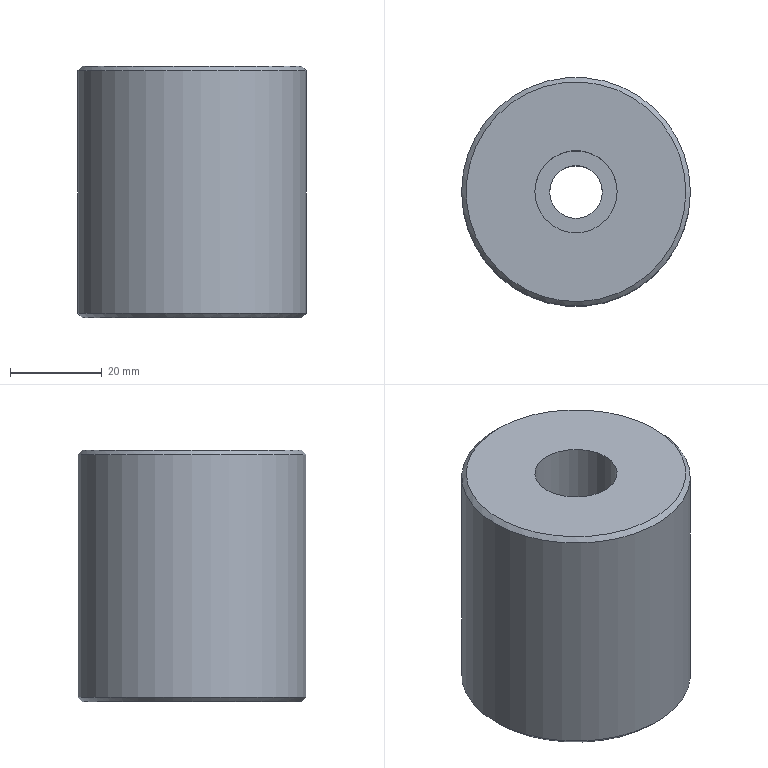Part | NX | features LB-2 2 | 1 solid | 8 faces | box 50 x 50 x 55 mm | volume 98356 mm3 | plane 3 | cylinder 3 | cone 2 | commonest cylinder face diameters 11.507 x1 18 x1 50 x1
STEP:
#1=CARTESIAN_POINT('',(3649.094,-666.122,858.717));
#2=VERTEX_POINT('',#1);
#3=CARTESIAN_POINT('',(3625.094,-666.122,858.717));
#4=DIRECTION('',(0.,0.,-1.));
#5=DIRECTION('',(1.,0.,0.));
#6=AXIS2_PLACEMENT_3D('',#3,#4,#5);
#7=CIRCLE('',#6,24.);
#8=EDGE_CURVE('',#2,#2,#7,.T.);
#9=ORIENTED_EDGE('',*,*,#8,.F.);
#10=EDGE_LOOP('',(#9));
#11=FACE_BOUND('',#10,.T.);
#12=CARTESIAN_POINT('',(3634.094,-666.122,858.717));
#13=VERTEX_POINT('',#12);
#14=CARTESIAN_POINT('',(3625.094,-666.122,858.717));
#15=DIRECTION('',(0.,0.,1.));
#16=DIRECTION('',(1.,0.,0.));
#17=AXIS2_PLACEMENT_3D('',#14,#15,#16);
#18=CIRCLE('',#17,9.);
#19=EDGE_CURVE('',#13,#13,#18,.T.);
#20=ORIENTED_EDGE('',*,*,#19,.F.);
#21=EDGE_LOOP('',(#20));
#22=FACE_BOUND('',#21,.T.);
#23=CARTESIAN_POINT('',(3625.094,-666.122,858.717));
#24=DIRECTION('',(0.,0.,1.));
#25=DIRECTION('',(-1.,0.,0.));
#26=AXIS2_PLACEMENT_3D('',#23,#24,#25);
#27=PLANE('',#26);
#28=ADVANCED_FACE('',(#11,#22),#27,.T.);
#29=CARTESIAN_POINT('',(3601.094,-666.122,803.716));
#30=VERTEX_POINT('',#29);
#31=CARTESIAN_POINT('',(3625.094,-666.122,803.716));
#32=DIRECTION('',(0.,0.,1.));
#33=DIRECTION('',(-1.,0.,0.));
#34=AXIS2_PLACEMENT_3D('',#31,#32,#33);
#35=CIRCLE('',#34,24.);
#36=EDGE_CURVE('',#30,#30,#35,.T.);
#37=ORIENTED_EDGE('',*,*,#36,.F.);
#38=EDGE_LOOP('',(#37));
#39=FACE_BOUND('',#38,.T.);
#40=CARTESIAN_POINT('',(3630.847,-666.122,803.716));
#41=VERTEX_POINT('',#40);
#42=CARTESIAN_POINT('',(3625.094,-666.122,803.716));
#43=DIRECTION('',(0.,0.,1.));
#44=DIRECTION('',(1.,0.,0.));
#45=AXIS2_PLACEMENT_3D('',#42,#43,#44);
#46=CIRCLE('',#45,5.753);
#47=EDGE_CURVE('',#41,#41,#46,.F.);
#48=ORIENTED_EDGE('',*,*,#47,.F.);
#49=EDGE_LOOP('',(#48));
#50=FACE_BOUND('',#49,.T.);
#51=CARTESIAN_POINT('',(3798.441,-854.122,803.716));
#52=DIRECTION('',(0.,0.,1.));
#53=DIRECTION('',(-1.,0.,0.));
#54=AXIS2_PLACEMENT_3D('',#51,#52,#53);
#55=PLANE('',#54);
#56=ADVANCED_FACE('',(#39,#50),#55,.F.);
#57=CARTESIAN_POINT('',(3650.094,-666.122,857.717));
#58=VERTEX_POINT('',#57);
#59=CARTESIAN_POINT('',(3625.094,-666.122,857.717));
#60=DIRECTION('',(0.,0.,1.));
#61=DIRECTION('',(1.,0.,0.));
#62=AXIS2_PLACEMENT_3D('',#59,#60,#61);
#63=CIRCLE('',#62,25.);
#64=EDGE_CURVE('',#58,#58,#63,.T.);
#65=ORIENTED_EDGE('',*,*,#64,.F.);
#66=EDGE_LOOP('',(#65));
#67=FACE_BOUND('',#66,.T.);
#68=CARTESIAN_POINT('',(3600.094,-666.122,804.716));
#69=VERTEX_POINT('',#68);
#70=CARTESIAN_POINT('',(3625.094,-666.122,804.716));
#71=DIRECTION('',(0.,0.,-1.));
#72=DIRECTION('',(-1.,0.,0.));
#73=AXIS2_PLACEMENT_3D('',#70,#71,#72);
#74=CIRCLE('',#73,25.);
#75=EDGE_CURVE('',#69,#69,#74,.T.);
#76=ORIENTED_EDGE('',*,*,#75,.F.);
#77=EDGE_LOOP('',(#76));
#78=FACE_BOUND('',#77,.T.);
#79=CARTESIAN_POINT('',(3625.094,-666.122,803.617));
#80=DIRECTION('',(0.,0.,1.));
#81=DIRECTION('',(-1.,0.,0.));
#82=AXIS2_PLACEMENT_3D('',#79,#80,#81);
#83=CYLINDRICAL_SURFACE('',#82,25.);
#84=ADVANCED_FACE('',(#67,#78),#83,.T.);
#85=CARTESIAN_POINT('',(3619.34,-666.122,833.717));
#86=VERTEX_POINT('',#85);
#87=CARTESIAN_POINT('',(3625.094,-666.122,833.717));
#88=DIRECTION('',(0.,0.,-1.));
#89=DIRECTION('',(-1.,0.,0.));
#90=AXIS2_PLACEMENT_3D('',#87,#88,#89);
#91=CIRCLE('',#90,5.753);
#92=EDGE_CURVE('',#86,#86,#91,.T.);
#93=ORIENTED_EDGE('',*,*,#92,.F.);
#94=EDGE_LOOP('',(#93));
#95=FACE_BOUND('',#94,.T.);
#96=ORIENTED_EDGE('',*,*,#47,.T.);
#97=EDGE_LOOP('',(#96));
#98=FACE_BOUND('',#97,.T.);
#99=CARTESIAN_POINT('',(3625.094,-666.122,803.617));
#100=DIRECTION('',(0.,0.,1.));
#101=DIRECTION('',(-1.,0.,0.));
#102=AXIS2_PLACEMENT_3D('',#99,#100,#101);
#103=CYLINDRICAL_SURFACE('',#102,5.753);
#104=ADVANCED_FACE('',(#95,#98),#103,.F.);
#105=CARTESIAN_POINT('',(3634.094,-666.122,833.717));
#106=VERTEX_POINT('',#105);
#107=CARTESIAN_POINT('',(3625.094,-666.122,833.717));
#108=DIRECTION('',(0.,0.,1.));
#109=DIRECTION('',(1.,0.,0.));
#110=AXIS2_PLACEMENT_3D('',#107,#108,#109);
#111=CIRCLE('',#110,9.);
#112=EDGE_CURVE('',#106,#106,#111,.T.);
#113=ORIENTED_EDGE('',*,*,#112,.T.);
#114=EDGE_LOOP('',(#113));
#115=FACE_BOUND('',#114,.T.);
#116=ORIENTED_EDGE('',*,*,#92,.T.);
#117=EDGE_LOOP('',(#116));
#118=FACE_BOUND('',#117,.T.);
#119=CARTESIAN_POINT('',(3625.094,-666.122,833.717));
#120=DIRECTION('',(0.,0.,-1.));
#121=DIRECTION('',(1.,0.,0.));
#122=AXIS2_PLACEMENT_3D('',#119,#120,#121);
#123=PLANE('',#122);
#124=ADVANCED_FACE('',(#115,#118),#123,.F.);
#125=ORIENTED_EDGE('',*,*,#19,.T.);
#126=EDGE_LOOP('',(#125));
#127=FACE_BOUND('',#126,.T.);
#128=ORIENTED_EDGE('',*,*,#112,.F.);
#129=EDGE_LOOP('',(#128));
#130=FACE_BOUND('',#129,.T.);
#131=CARTESIAN_POINT('',(3625.094,-666.122,833.717));
#132=DIRECTION('',(0.,0.,1.));
#133=DIRECTION('',(-1.,0.,0.));
#134=AXIS2_PLACEMENT_3D('',#131,#132,#133);
#135=CYLINDRICAL_SURFACE('',#134,9.);
#136=ADVANCED_FACE('',(#127,#130),#135,.F.);
#137=ORIENTED_EDGE('',*,*,#8,.T.);
#138=EDGE_LOOP('',(#137));
#139=FACE_BOUND('',#138,.T.);
#140=ORIENTED_EDGE('',*,*,#64,.T.);
#141=EDGE_LOOP('',(#140));
#142=FACE_BOUND('',#141,.T.);
#143=CARTESIAN_POINT('',(3625.094,-666.122,857.717));
#144=DIRECTION('',(0.,0.,-1.));
#145=DIRECTION('',(1.,0.,0.));
#146=AXIS2_PLACEMENT_3D('',#143,#144,#145);
#147=CONICAL_SURFACE('',#146,25.,0.7854);
#148=ADVANCED_FACE('',(#139,#142),#147,.T.);
#149=ORIENTED_EDGE('',*,*,#36,.T.);
#150=EDGE_LOOP('',(#149));
#151=FACE_BOUND('',#150,.T.);
#152=ORIENTED_EDGE('',*,*,#75,.T.);
#153=EDGE_LOOP('',(#152));
#154=FACE_BOUND('',#153,.T.);
#155=CARTESIAN_POINT('',(3625.094,-666.122,804.716));
#156=DIRECTION('',(0.,0.,1.));
#157=DIRECTION('',(1.,0.,0.));
#158=AXIS2_PLACEMENT_3D('',#155,#156,#157);
#159=CONICAL_SURFACE('',#158,25.,0.7854);
#160=ADVANCED_FACE('',(#151,#154),#159,.T.);
#161=CLOSED_SHELL('',(#28,#56,#84,#104,#124,#136,#148,#160));
#162=MANIFOLD_SOLID_BREP('',#161);
#163=(LENGTH_UNIT()NAMED_UNIT(*)SI_UNIT(.MILLI.,.METRE.));
#164=UNCERTAINTY_MEASURE_WITH_UNIT(LENGTH_MEASURE(0.00001),#163,'','');
#165=(NAMED_UNIT(*)PLANE_ANGLE_UNIT()SI_UNIT($,.RADIAN.));
#166=(NAMED_UNIT(*)SI_UNIT($,.STERADIAN.)SOLID_ANGLE_UNIT());
#167=(GEOMETRIC_REPRESENTATION_CONTEXT(3)GLOBAL_UNCERTAINTY_ASSIGNED_CONTEXT((#164))GLOBAL_UNIT_ASSIGNED_CONTEXT((#163,#165,#166))REPRESENTATION_CONTEXT('',''));
#168=ADVANCED_BREP_SHAPE_REPRESENTATION('',(#162),#167);